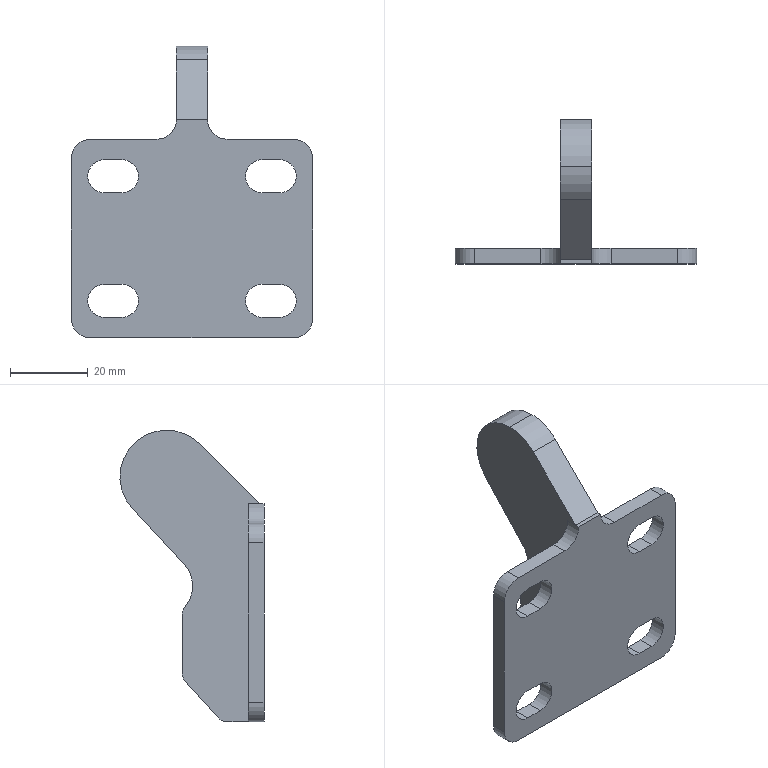Part | STEP file | _1-QC-408710.step | 1 solid | 43 faces | box 62 x 37 x 74.9 mm | volume 22748 mm3 | plane 23 | cylinder 20 | commonest cylinder face diameters 8.5 x8 10 x6 6 x3 24 x2 16 x1